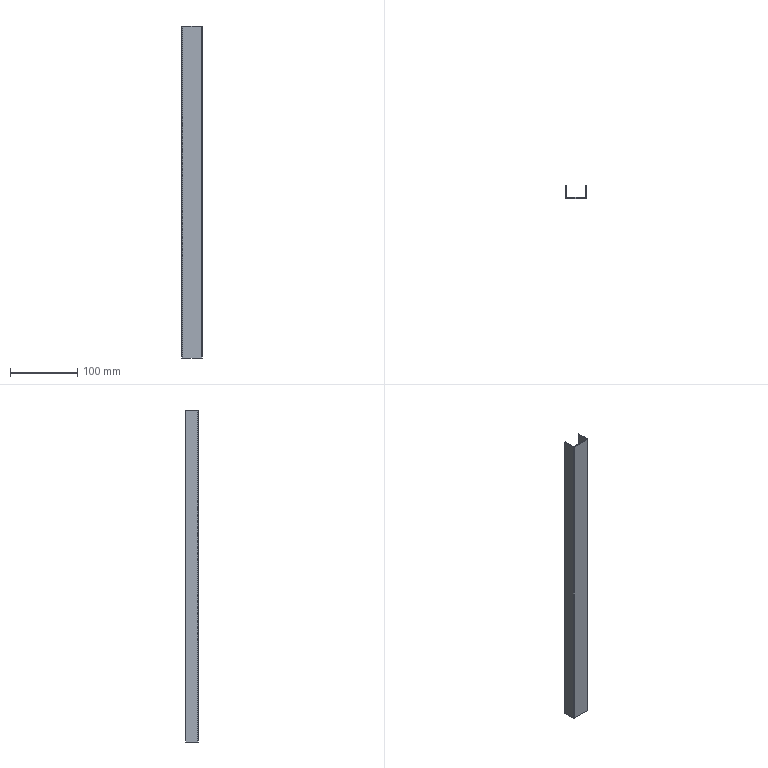Part | SolidWorks | features SplitBody 1 | 1 solid | 22 faces | box 30 x 19 x 495 mm | volume 32415 mm3 | plane 18 | cylinder 4 | commonest cylinder face diameters 0.2 x2 2.2 x2
STEP:
#1=CARTESIAN_POINT('',(-13.9,1595.5,-247.5));
#2=VERTEX_POINT('',#1);
#3=CARTESIAN_POINT('',(-13.9,1596.5,-247.5));
#4=VERTEX_POINT('',#3);
#5=CARTESIAN_POINT('',(-13.9,1595.5,-247.5));
#6=DIRECTION('',(0.,1.,0.));
#7=VECTOR('',#6,1000.);
#8=LINE('',#5,#7);
#9=EDGE_CURVE('',#2,#4,#8,.T.);
#10=ORIENTED_EDGE('',*,*,#9,.F.);
#11=CARTESIAN_POINT('',(-15.,1596.6,-247.5));
#12=VERTEX_POINT('',#11);
#13=CARTESIAN_POINT('',(-13.9,1596.6,-247.5));
#14=DIRECTION('',(0.,0.,1.));
#15=DIRECTION('',(-1.,0.,0.));
#16=AXIS2_PLACEMENT_3D('',#13,#14,#15);
#17=CIRCLE('',#16,1.1);
#18=EDGE_CURVE('',#12,#2,#17,.T.);
#19=ORIENTED_EDGE('',*,*,#18,.F.);
#20=CARTESIAN_POINT('',(-14.,1596.6,-247.5));
#21=VERTEX_POINT('',#20);
#22=CARTESIAN_POINT('',(-14.,1596.6,-247.5));
#23=DIRECTION('',(-1.,0.,0.));
#24=VECTOR('',#23,1000.);
#25=LINE('',#22,#24);
#26=EDGE_CURVE('',#21,#12,#25,.T.);
#27=ORIENTED_EDGE('',*,*,#26,.F.);
#28=CARTESIAN_POINT('',(-13.9,1596.6,-247.5));
#29=DIRECTION('',(0.,0.,1.));
#30=DIRECTION('',(1.,0.,0.));
#31=AXIS2_PLACEMENT_3D('',#28,#29,#30);
#32=CIRCLE('',#31,0.1);
#33=EDGE_CURVE('',#21,#4,#32,.T.);
#34=ORIENTED_EDGE('',*,*,#33,.T.);
#35=EDGE_LOOP('',(#10,#19,#27,#34));
#36=FACE_OUTER_BOUND('',#35,.T.);
#37=CARTESIAN_POINT('',(-13.9,1595.5,-247.5));
#38=DIRECTION('',(0.,0.,-1.));
#39=DIRECTION('',(-1.,0.,0.));
#40=AXIS2_PLACEMENT_3D('',#37,#38,#39);
#41=PLANE('',#40);
#42=ADVANCED_FACE('',(#36),#41,.T.);
#43=CARTESIAN_POINT('',(13.9,1595.5,-247.5));
#44=VERTEX_POINT('',#43);
#45=CARTESIAN_POINT('',(-15.,1595.5,-247.5));
#46=DIRECTION('',(1.,0.,0.));
#47=VECTOR('',#46,1000.);
#48=LINE('',#45,#47);
#49=EDGE_CURVE('',#2,#44,#48,.T.);
#50=ORIENTED_EDGE('',*,*,#49,.F.);
#51=ORIENTED_EDGE('',*,*,#9,.T.);
#52=CARTESIAN_POINT('',(13.9,1596.5,-247.5));
#53=VERTEX_POINT('',#52);
#54=CARTESIAN_POINT('',(-15.,1596.5,-247.5));
#55=DIRECTION('',(1.,0.,0.));
#56=VECTOR('',#55,1000.);
#57=LINE('',#54,#56);
#58=EDGE_CURVE('',#4,#53,#57,.T.);
#59=ORIENTED_EDGE('',*,*,#58,.T.);
#60=CARTESIAN_POINT('',(13.9,1596.5,-247.5));
#61=DIRECTION('',(0.,-1.,0.));
#62=VECTOR('',#61,1000.);
#63=LINE('',#60,#62);
#64=EDGE_CURVE('',#53,#44,#63,.T.);
#65=ORIENTED_EDGE('',*,*,#64,.T.);
#66=EDGE_LOOP('',(#50,#51,#59,#65));
#67=FACE_OUTER_BOUND('',#66,.T.);
#68=CARTESIAN_POINT('',(-14.,1596.6,-247.5));
#69=DIRECTION('',(0.,0.,-1.));
#70=DIRECTION('',(-1.,0.,0.));
#71=AXIS2_PLACEMENT_3D('',#68,#69,#70);
#72=PLANE('',#71);
#73=ADVANCED_FACE('',(#67),#72,.T.);
#74=CARTESIAN_POINT('',(15.,1596.6,-247.5));
#75=VERTEX_POINT('',#74);
#76=CARTESIAN_POINT('',(14.,1596.6,-247.5));
#77=VERTEX_POINT('',#76);
#78=CARTESIAN_POINT('',(15.,1596.6,-247.5));
#79=DIRECTION('',(-1.,0.,0.));
#80=VECTOR('',#79,1000.);
#81=LINE('',#78,#80);
#82=EDGE_CURVE('',#75,#77,#81,.T.);
#83=ORIENTED_EDGE('',*,*,#82,.F.);
#84=CARTESIAN_POINT('',(13.9,1596.6,-247.5));
#85=DIRECTION('',(0.,0.,1.));
#86=DIRECTION('',(-1.,0.,0.));
#87=AXIS2_PLACEMENT_3D('',#84,#85,#86);
#88=CIRCLE('',#87,1.1);
#89=EDGE_CURVE('',#44,#75,#88,.T.);
#90=ORIENTED_EDGE('',*,*,#89,.F.);
#91=ORIENTED_EDGE('',*,*,#64,.F.);
#92=CARTESIAN_POINT('',(13.9,1596.6,-247.5));
#93=DIRECTION('',(0.,0.,1.));
#94=DIRECTION('',(1.,0.,0.));
#95=AXIS2_PLACEMENT_3D('',#92,#93,#94);
#96=CIRCLE('',#95,0.1);
#97=EDGE_CURVE('',#53,#77,#96,.T.);
#98=ORIENTED_EDGE('',*,*,#97,.T.);
#99=EDGE_LOOP('',(#83,#90,#91,#98));
#100=FACE_OUTER_BOUND('',#99,.T.);
#101=CARTESIAN_POINT('',(15.,1596.6,-247.5));
#102=DIRECTION('',(0.,0.,-1.));
#103=DIRECTION('',(-1.,0.,0.));
#104=AXIS2_PLACEMENT_3D('',#101,#102,#103);
#105=PLANE('',#104);
#106=ADVANCED_FACE('',(#100),#105,.T.);
#107=CARTESIAN_POINT('',(15.,1614.5,-247.5));
#108=VERTEX_POINT('',#107);
#109=CARTESIAN_POINT('',(15.,1595.5,-247.5));
#110=DIRECTION('',(0.,1.,0.));
#111=VECTOR('',#110,1000.);
#112=LINE('',#109,#111);
#113=EDGE_CURVE('',#75,#108,#112,.T.);
#114=ORIENTED_EDGE('',*,*,#113,.F.);
#115=ORIENTED_EDGE('',*,*,#82,.T.);
#116=CARTESIAN_POINT('',(14.,1614.5,-247.5));
#117=VERTEX_POINT('',#116);
#118=CARTESIAN_POINT('',(14.,1595.5,-247.5));
#119=DIRECTION('',(0.,1.,0.));
#120=VECTOR('',#119,1000.);
#121=LINE('',#118,#120);
#122=EDGE_CURVE('',#77,#117,#121,.T.);
#123=ORIENTED_EDGE('',*,*,#122,.T.);
#124=CARTESIAN_POINT('',(14.,1614.5,-247.5));
#125=DIRECTION('',(1.,0.,0.));
#126=VECTOR('',#125,1000.);
#127=LINE('',#124,#126);
#128=EDGE_CURVE('',#117,#108,#127,.T.);
#129=ORIENTED_EDGE('',*,*,#128,.T.);
#130=EDGE_LOOP('',(#114,#115,#123,#129));
#131=FACE_OUTER_BOUND('',#130,.T.);
#132=CARTESIAN_POINT('',(13.9,1596.5,-247.5));
#133=DIRECTION('',(0.,0.,-1.));
#134=DIRECTION('',(-1.,0.,0.));
#135=AXIS2_PLACEMENT_3D('',#132,#133,#134);
#136=PLANE('',#135);
#137=ADVANCED_FACE('',(#131),#136,.T.);
#138=CARTESIAN_POINT('',(15.,1614.5,247.5));
#139=VERTEX_POINT('',#138);
#140=CARTESIAN_POINT('',(15.,1596.6,247.5));
#141=VERTEX_POINT('',#140);
#142=CARTESIAN_POINT('',(15.,1595.5,247.5));
#143=DIRECTION('',(0.,-1.,0.));
#144=VECTOR('',#143,1000.);
#145=LINE('',#142,#144);
#146=EDGE_CURVE('',#139,#141,#145,.T.);
#147=ORIENTED_EDGE('',*,*,#146,.T.);
#148=CARTESIAN_POINT('',(15.,1596.6,283.011));
#149=DIRECTION('',(0.,0.,-1.));
#150=VECTOR('',#149,1000.);
#151=LINE('',#148,#150);
#152=EDGE_CURVE('',#141,#75,#151,.T.);
#153=ORIENTED_EDGE('',*,*,#152,.T.);
#154=ORIENTED_EDGE('',*,*,#113,.T.);
#155=CARTESIAN_POINT('',(15.,1614.5,283.011));
#156=DIRECTION('',(0.,0.,-1.));
#157=VECTOR('',#156,1000.);
#158=LINE('',#155,#157);
#159=EDGE_CURVE('',#139,#108,#158,.T.);
#160=ORIENTED_EDGE('',*,*,#159,.F.);
#161=EDGE_LOOP('',(#147,#153,#154,#160));
#162=FACE_OUTER_BOUND('',#161,.T.);
#163=CARTESIAN_POINT('',(15.,1595.5,283.011));
#164=DIRECTION('',(-1.,0.,0.));
#165=DIRECTION('',(0.,-1.,0.));
#166=AXIS2_PLACEMENT_3D('',#163,#164,#165);
#167=PLANE('',#166);
#168=ADVANCED_FACE('',(#162),#167,.F.);
#169=CARTESIAN_POINT('',(14.,1614.5,247.5));
#170=VERTEX_POINT('',#169);
#171=CARTESIAN_POINT('',(14.,1614.5,283.011));
#172=DIRECTION('',(0.,0.,-1.));
#173=VECTOR('',#172,1000.);
#174=LINE('',#171,#173);
#175=EDGE_CURVE('',#170,#117,#174,.T.);
#176=ORIENTED_EDGE('',*,*,#175,.F.);
#177=CARTESIAN_POINT('',(15.,1614.5,247.5));
#178=DIRECTION('',(-1.,0.,0.));
#179=VECTOR('',#178,1000.);
#180=LINE('',#177,#179);
#181=EDGE_CURVE('',#139,#170,#180,.T.);
#182=ORIENTED_EDGE('',*,*,#181,.F.);
#183=ORIENTED_EDGE('',*,*,#159,.T.);
#184=ORIENTED_EDGE('',*,*,#128,.F.);
#185=EDGE_LOOP('',(#176,#182,#183,#184));
#186=FACE_OUTER_BOUND('',#185,.T.);
#187=CARTESIAN_POINT('',(14.,1614.5,283.011));
#188=DIRECTION('',(0.,1.,0.));
#189=DIRECTION('',(0.,0.,1.));
#190=AXIS2_PLACEMENT_3D('',#187,#188,#189);
#191=PLANE('',#190);
#192=ADVANCED_FACE('',(#186),#191,.T.);
#193=CARTESIAN_POINT('',(14.,1596.6,247.5));
#194=VERTEX_POINT('',#193);
#195=CARTESIAN_POINT('',(14.,1596.6,283.011));
#196=DIRECTION('',(0.,0.,-1.));
#197=VECTOR('',#196,1000.);
#198=LINE('',#195,#197);
#199=EDGE_CURVE('',#194,#77,#198,.T.);
#200=ORIENTED_EDGE('',*,*,#199,.F.);
#201=CARTESIAN_POINT('',(14.,1595.5,247.5));
#202=DIRECTION('',(0.,-1.,0.));
#203=VECTOR('',#202,1000.);
#204=LINE('',#201,#203);
#205=EDGE_CURVE('',#170,#194,#204,.T.);
#206=ORIENTED_EDGE('',*,*,#205,.F.);
#207=ORIENTED_EDGE('',*,*,#175,.T.);
#208=ORIENTED_EDGE('',*,*,#122,.F.);
#209=EDGE_LOOP('',(#200,#206,#207,#208));
#210=FACE_OUTER_BOUND('',#209,.T.);
#211=CARTESIAN_POINT('',(14.,1595.5,283.011));
#212=DIRECTION('',(-1.,0.,0.));
#213=DIRECTION('',(0.,-1.,0.));
#214=AXIS2_PLACEMENT_3D('',#211,#212,#213);
#215=PLANE('',#214);
#216=ADVANCED_FACE('',(#210),#215,.T.);
#217=CARTESIAN_POINT('',(13.9,1596.5,247.5));
#218=VERTEX_POINT('',#217);
#219=CARTESIAN_POINT('',(13.9,1596.5,283.011));
#220=DIRECTION('',(0.,0.,-1.));
#221=VECTOR('',#220,1000.);
#222=LINE('',#219,#221);
#223=EDGE_CURVE('',#218,#53,#222,.T.);
#224=ORIENTED_EDGE('',*,*,#223,.F.);
#225=CARTESIAN_POINT('',(13.9,1596.6,247.5));
#226=DIRECTION('',(0.,0.,-1.));
#227=DIRECTION('',(1.,0.,0.));
#228=AXIS2_PLACEMENT_3D('',#225,#226,#227);
#229=CIRCLE('',#228,0.1);
#230=EDGE_CURVE('',#194,#218,#229,.T.);
#231=ORIENTED_EDGE('',*,*,#230,.F.);
#232=ORIENTED_EDGE('',*,*,#199,.T.);
#233=ORIENTED_EDGE('',*,*,#97,.F.);
#234=EDGE_LOOP('',(#224,#231,#232,#233));
#235=FACE_OUTER_BOUND('',#234,.T.);
#236=CARTESIAN_POINT('',(13.9,1596.6,283.011));
#237=DIRECTION('',(0.,0.,-1.));
#238=DIRECTION('',(-1.,0.,0.));
#239=AXIS2_PLACEMENT_3D('',#236,#237,#238);
#240=CYLINDRICAL_SURFACE('',#239,0.1);
#241=ADVANCED_FACE('',(#235),#240,.F.);
#242=CARTESIAN_POINT('',(-13.9,1596.5,247.5));
#243=VERTEX_POINT('',#242);
#244=CARTESIAN_POINT('',(-13.9,1596.5,283.011));
#245=DIRECTION('',(0.,0.,-1.));
#246=VECTOR('',#245,1000.);
#247=LINE('',#244,#246);
#248=EDGE_CURVE('',#243,#4,#247,.T.);
#249=ORIENTED_EDGE('',*,*,#248,.F.);
#250=CARTESIAN_POINT('',(-15.,1596.5,247.5));
#251=DIRECTION('',(-1.,0.,0.));
#252=VECTOR('',#251,1000.);
#253=LINE('',#250,#252);
#254=EDGE_CURVE('',#218,#243,#253,.T.);
#255=ORIENTED_EDGE('',*,*,#254,.F.);
#256=ORIENTED_EDGE('',*,*,#223,.T.);
#257=ORIENTED_EDGE('',*,*,#58,.F.);
#258=EDGE_LOOP('',(#249,#255,#256,#257));
#259=FACE_OUTER_BOUND('',#258,.T.);
#260=CARTESIAN_POINT('',(-15.,1596.5,283.011));
#261=DIRECTION('',(0.,1.,0.));
#262=DIRECTION('',(0.,0.,1.));
#263=AXIS2_PLACEMENT_3D('',#260,#261,#262);
#264=PLANE('',#263);
#265=ADVANCED_FACE('',(#259),#264,.T.);
#266=CARTESIAN_POINT('',(-14.,1596.6,247.5));
#267=VERTEX_POINT('',#266);
#268=CARTESIAN_POINT('',(-14.,1596.6,283.011));
#269=DIRECTION('',(0.,0.,-1.));
#270=VECTOR('',#269,1000.);
#271=LINE('',#268,#270);
#272=EDGE_CURVE('',#267,#21,#271,.T.);
#273=ORIENTED_EDGE('',*,*,#272,.F.);
#274=CARTESIAN_POINT('',(-13.9,1596.6,247.5));
#275=DIRECTION('',(0.,0.,-1.));
#276=DIRECTION('',(1.,0.,0.));
#277=AXIS2_PLACEMENT_3D('',#274,#275,#276);
#278=CIRCLE('',#277,0.1);
#279=EDGE_CURVE('',#243,#267,#278,.T.);
#280=ORIENTED_EDGE('',*,*,#279,.F.);
#281=ORIENTED_EDGE('',*,*,#248,.T.);
#282=ORIENTED_EDGE('',*,*,#33,.F.);
#283=EDGE_LOOP('',(#273,#280,#281,#282));
#284=FACE_OUTER_BOUND('',#283,.T.);
#285=CARTESIAN_POINT('',(-13.9,1596.6,283.011));
#286=DIRECTION('',(0.,0.,-1.));
#287=DIRECTION('',(-1.,0.,0.));
#288=AXIS2_PLACEMENT_3D('',#285,#286,#287);
#289=CYLINDRICAL_SURFACE('',#288,0.1);
#290=ADVANCED_FACE('',(#284),#289,.F.);
#291=CARTESIAN_POINT('',(-14.,1614.5,247.5));
#292=VERTEX_POINT('',#291);
#293=CARTESIAN_POINT('',(-14.,1614.5,-247.5));
#294=VERTEX_POINT('',#293);
#295=CARTESIAN_POINT('',(-14.,1614.5,283.011));
#296=DIRECTION('',(0.,0.,-1.));
#297=VECTOR('',#296,1000.);
#298=LINE('',#295,#297);
#299=EDGE_CURVE('',#292,#294,#298,.T.);
#300=ORIENTED_EDGE('',*,*,#299,.F.);
#301=CARTESIAN_POINT('',(-14.,1614.5,247.5));
#302=DIRECTION('',(0.,1.,0.));
#303=VECTOR('',#302,1000.);
#304=LINE('',#301,#303);
#305=EDGE_CURVE('',#267,#292,#304,.T.);
#306=ORIENTED_EDGE('',*,*,#305,.F.);
#307=ORIENTED_EDGE('',*,*,#272,.T.);
#308=CARTESIAN_POINT('',(-14.,1614.5,-247.5));
#309=DIRECTION('',(0.,-1.,0.));
#310=VECTOR('',#309,1000.);
#311=LINE('',#308,#310);
#312=EDGE_CURVE('',#294,#21,#311,.T.);
#313=ORIENTED_EDGE('',*,*,#312,.F.);
#314=EDGE_LOOP('',(#300,#306,#307,#313));
#315=FACE_OUTER_BOUND('',#314,.T.);
#316=CARTESIAN_POINT('',(-14.,1614.5,283.011));
#317=DIRECTION('',(1.,0.,0.));
#318=DIRECTION('',(0.,1.,0.));
#319=AXIS2_PLACEMENT_3D('',#316,#317,#318);
#320=PLANE('',#319);
#321=ADVANCED_FACE('',(#315),#320,.T.);
#322=CARTESIAN_POINT('',(-15.,1614.5,247.5));
#323=VERTEX_POINT('',#322);
#324=CARTESIAN_POINT('',(-15.,1614.5,-247.5));
#325=VERTEX_POINT('',#324);
#326=CARTESIAN_POINT('',(-15.,1614.5,283.011));
#327=DIRECTION('',(0.,0.,-1.));
#328=VECTOR('',#327,1000.);
#329=LINE('',#326,#328);
#330=EDGE_CURVE('',#323,#325,#329,.T.);
#331=ORIENTED_EDGE('',*,*,#330,.F.);
#332=CARTESIAN_POINT('',(-15.,1614.5,247.5));
#333=DIRECTION('',(1.,0.,0.));
#334=VECTOR('',#333,1000.);
#335=LINE('',#332,#334);
#336=EDGE_CURVE('',#323,#292,#335,.T.);
#337=ORIENTED_EDGE('',*,*,#336,.T.);
#338=ORIENTED_EDGE('',*,*,#299,.T.);
#339=CARTESIAN_POINT('',(-15.,1614.5,-247.5));
#340=DIRECTION('',(1.,0.,0.));
#341=VECTOR('',#340,1000.);
#342=LINE('',#339,#341);
#343=EDGE_CURVE('',#325,#294,#342,.T.);
#344=ORIENTED_EDGE('',*,*,#343,.F.);
#345=EDGE_LOOP('',(#331,#337,#338,#344));
#346=FACE_OUTER_BOUND('',#345,.T.);
#347=CARTESIAN_POINT('',(-15.,1614.5,283.011));
#348=DIRECTION('',(0.,1.,0.));
#349=DIRECTION('',(0.,0.,1.));
#350=AXIS2_PLACEMENT_3D('',#347,#348,#349);
#351=PLANE('',#350);
#352=ADVANCED_FACE('',(#346),#351,.T.);
#353=CARTESIAN_POINT('',(-15.,1596.6,247.5));
#354=VERTEX_POINT('',#353);
#355=CARTESIAN_POINT('',(-15.,1614.5,247.5));
#356=DIRECTION('',(0.,1.,0.));
#357=VECTOR('',#356,1000.);
#358=LINE('',#355,#357);
#359=EDGE_CURVE('',#354,#323,#358,.T.);
#360=ORIENTED_EDGE('',*,*,#359,.T.);
#361=ORIENTED_EDGE('',*,*,#330,.T.);
#362=CARTESIAN_POINT('',(-15.,1614.5,-247.5));
#363=DIRECTION('',(0.,-1.,0.));
#364=VECTOR('',#363,1000.);
#365=LINE('',#362,#364);
#366=EDGE_CURVE('',#325,#12,#365,.T.);
#367=ORIENTED_EDGE('',*,*,#366,.T.);
#368=CARTESIAN_POINT('',(-15.,1596.6,283.011));
#369=DIRECTION('',(0.,0.,-1.));
#370=VECTOR('',#369,1000.);
#371=LINE('',#368,#370);
#372=EDGE_CURVE('',#354,#12,#371,.T.);
#373=ORIENTED_EDGE('',*,*,#372,.F.);
#374=EDGE_LOOP('',(#360,#361,#367,#373));
#375=FACE_OUTER_BOUND('',#374,.T.);
#376=CARTESIAN_POINT('',(-15.,1614.5,283.011));
#377=DIRECTION('',(1.,0.,0.));
#378=DIRECTION('',(0.,1.,0.));
#379=AXIS2_PLACEMENT_3D('',#376,#377,#378);
#380=PLANE('',#379);
#381=ADVANCED_FACE('',(#375),#380,.F.);
#382=CARTESIAN_POINT('',(-13.9,1595.5,247.5));
#383=VERTEX_POINT('',#382);
#384=CARTESIAN_POINT('',(-13.9,1596.6,247.5));
#385=DIRECTION('',(0.,0.,-1.));
#386=DIRECTION('',(-1.,0.,0.));
#387=AXIS2_PLACEMENT_3D('',#384,#385,#386);
#388=CIRCLE('',#387,1.1);
#389=EDGE_CURVE('',#383,#354,#388,.T.);
#390=ORIENTED_EDGE('',*,*,#389,.T.);
#391=ORIENTED_EDGE('',*,*,#372,.T.);
#392=ORIENTED_EDGE('',*,*,#18,.T.);
#393=CARTESIAN_POINT('',(-13.9,1595.5,283.011));
#394=DIRECTION('',(0.,0.,-1.));
#395=VECTOR('',#394,1000.);
#396=LINE('',#393,#395);
#397=EDGE_CURVE('',#383,#2,#396,.T.);
#398=ORIENTED_EDGE('',*,*,#397,.F.);
#399=EDGE_LOOP('',(#390,#391,#392,#398));
#400=FACE_OUTER_BOUND('',#399,.T.);
#401=CARTESIAN_POINT('',(-13.9,1596.6,283.011));
#402=DIRECTION('',(0.,0.,-1.));
#403=DIRECTION('',(-1.,0.,0.));
#404=AXIS2_PLACEMENT_3D('',#401,#402,#403);
#405=CYLINDRICAL_SURFACE('',#404,1.1);
#406=ADVANCED_FACE('',(#400),#405,.T.);
#407=CARTESIAN_POINT('',(13.9,1595.5,247.5));
#408=VERTEX_POINT('',#407);
#409=CARTESIAN_POINT('',(-15.,1595.5,247.5));
#410=DIRECTION('',(-1.,0.,0.));
#411=VECTOR('',#410,1000.);
#412=LINE('',#409,#411);
#413=EDGE_CURVE('',#408,#383,#412,.T.);
#414=ORIENTED_EDGE('',*,*,#413,.T.);
#415=ORIENTED_EDGE('',*,*,#397,.T.);
#416=ORIENTED_EDGE('',*,*,#49,.T.);
#417=CARTESIAN_POINT('',(13.9,1595.5,283.011));
#418=DIRECTION('',(0.,0.,-1.));
#419=VECTOR('',#418,1000.);
#420=LINE('',#417,#419);
#421=EDGE_CURVE('',#408,#44,#420,.T.);
#422=ORIENTED_EDGE('',*,*,#421,.F.);
#423=EDGE_LOOP('',(#414,#415,#416,#422));
#424=FACE_OUTER_BOUND('',#423,.T.);
#425=CARTESIAN_POINT('',(-15.,1595.5,283.011));
#426=DIRECTION('',(0.,1.,0.));
#427=DIRECTION('',(0.,0.,1.));
#428=AXIS2_PLACEMENT_3D('',#425,#426,#427);
#429=PLANE('',#428);
#430=ADVANCED_FACE('',(#424),#429,.F.);
#431=CARTESIAN_POINT('',(13.9,1596.6,247.5));
#432=DIRECTION('',(0.,0.,-1.));
#433=DIRECTION('',(-1.,0.,0.));
#434=AXIS2_PLACEMENT_3D('',#431,#432,#433);
#435=CIRCLE('',#434,1.1);
#436=EDGE_CURVE('',#141,#408,#435,.T.);
#437=ORIENTED_EDGE('',*,*,#436,.T.);
#438=ORIENTED_EDGE('',*,*,#421,.T.);
#439=ORIENTED_EDGE('',*,*,#89,.T.);
#440=ORIENTED_EDGE('',*,*,#152,.F.);
#441=EDGE_LOOP('',(#437,#438,#439,#440));
#442=FACE_OUTER_BOUND('',#441,.T.);
#443=CARTESIAN_POINT('',(13.9,1596.6,283.011));
#444=DIRECTION('',(0.,0.,-1.));
#445=DIRECTION('',(-1.,0.,0.));
#446=AXIS2_PLACEMENT_3D('',#443,#444,#445);
#447=CYLINDRICAL_SURFACE('',#446,1.1);
#448=ADVANCED_FACE('',(#442),#447,.T.);
#449=ORIENTED_EDGE('',*,*,#312,.T.);
#450=ORIENTED_EDGE('',*,*,#26,.T.);
#451=ORIENTED_EDGE('',*,*,#366,.F.);
#452=ORIENTED_EDGE('',*,*,#343,.T.);
#453=EDGE_LOOP('',(#449,#450,#451,#452));
#454=FACE_OUTER_BOUND('',#453,.T.);
#455=CARTESIAN_POINT('',(13.9,1596.6,-247.5));
#456=DIRECTION('',(0.,0.,1.));
#457=DIRECTION('',(1.,0.,0.));
#458=AXIS2_PLACEMENT_3D('',#455,#456,#457);
#459=PLANE('',#458);
#460=ADVANCED_FACE('',(#454),#459,.F.);
#461=CARTESIAN_POINT('',(15.,1596.6,247.5));
#462=DIRECTION('',(-1.,0.,0.));
#463=VECTOR('',#462,1000.);
#464=LINE('',#461,#463);
#465=EDGE_CURVE('',#141,#194,#464,.T.);
#466=ORIENTED_EDGE('',*,*,#465,.F.);
#467=ORIENTED_EDGE('',*,*,#146,.F.);
#468=ORIENTED_EDGE('',*,*,#181,.T.);
#469=ORIENTED_EDGE('',*,*,#205,.T.);
#470=EDGE_LOOP('',(#466,#467,#468,#469));
#471=FACE_OUTER_BOUND('',#470,.T.);
#472=CARTESIAN_POINT('',(15.,1595.5,247.5));
#473=DIRECTION('',(0.,0.,-1.));
#474=DIRECTION('',(0.,-1.,0.));
#475=AXIS2_PLACEMENT_3D('',#472,#473,#474);
#476=PLANE('',#475);
#477=ADVANCED_FACE('',(#471),#476,.F.);
#478=CARTESIAN_POINT('',(-13.9,1595.5,247.5));
#479=DIRECTION('',(0.,1.,0.));
#480=VECTOR('',#479,1000.);
#481=LINE('',#478,#480);
#482=EDGE_CURVE('',#383,#243,#481,.T.);
#483=ORIENTED_EDGE('',*,*,#482,.F.);
#484=ORIENTED_EDGE('',*,*,#413,.F.);
#485=CARTESIAN_POINT('',(13.9,1595.5,247.5));
#486=DIRECTION('',(0.,1.,0.));
#487=VECTOR('',#486,1000.);
#488=LINE('',#485,#487);
#489=EDGE_CURVE('',#408,#218,#488,.T.);
#490=ORIENTED_EDGE('',*,*,#489,.T.);
#491=ORIENTED_EDGE('',*,*,#254,.T.);
#492=EDGE_LOOP('',(#483,#484,#490,#491));
#493=FACE_OUTER_BOUND('',#492,.T.);
#494=CARTESIAN_POINT('',(-15.,1595.5,247.5));
#495=DIRECTION('',(0.,0.,-1.));
#496=DIRECTION('',(-1.,0.,0.));
#497=AXIS2_PLACEMENT_3D('',#494,#495,#496);
#498=PLANE('',#497);
#499=ADVANCED_FACE('',(#493),#498,.F.);
#500=ORIENTED_EDGE('',*,*,#336,.F.);
#501=ORIENTED_EDGE('',*,*,#359,.F.);
#502=CARTESIAN_POINT('',(-15.,1596.6,247.5));
#503=DIRECTION('',(1.,0.,0.));
#504=VECTOR('',#503,1000.);
#505=LINE('',#502,#504);
#506=EDGE_CURVE('',#354,#267,#505,.T.);
#507=ORIENTED_EDGE('',*,*,#506,.T.);
#508=ORIENTED_EDGE('',*,*,#305,.T.);
#509=EDGE_LOOP('',(#500,#501,#507,#508));
#510=FACE_OUTER_BOUND('',#509,.T.);
#511=CARTESIAN_POINT('',(-15.,1614.5,247.5));
#512=DIRECTION('',(0.,0.,-1.));
#513=DIRECTION('',(0.,1.,0.));
#514=AXIS2_PLACEMENT_3D('',#511,#512,#513);
#515=PLANE('',#514);
#516=ADVANCED_FACE('',(#510),#515,.F.);
#517=ORIENTED_EDGE('',*,*,#279,.T.);
#518=ORIENTED_EDGE('',*,*,#506,.F.);
#519=ORIENTED_EDGE('',*,*,#389,.F.);
#520=ORIENTED_EDGE('',*,*,#482,.T.);
#521=EDGE_LOOP('',(#517,#518,#519,#520));
#522=FACE_OUTER_BOUND('',#521,.T.);
#523=CARTESIAN_POINT('',(-13.9,1596.6,247.5));
#524=DIRECTION('',(0.,0.,1.));
#525=DIRECTION('',(1.,0.,0.));
#526=AXIS2_PLACEMENT_3D('',#523,#524,#525);
#527=PLANE('',#526);
#528=ADVANCED_FACE('',(#522),#527,.T.);
#529=ORIENTED_EDGE('',*,*,#230,.T.);
#530=ORIENTED_EDGE('',*,*,#489,.F.);
#531=ORIENTED_EDGE('',*,*,#436,.F.);
#532=ORIENTED_EDGE('',*,*,#465,.T.);
#533=EDGE_LOOP('',(#529,#530,#531,#532));
#534=FACE_OUTER_BOUND('',#533,.T.);
#535=CARTESIAN_POINT('',(13.9,1596.6,247.5));
#536=DIRECTION('',(0.,0.,1.));
#537=DIRECTION('',(1.,0.,0.));
#538=AXIS2_PLACEMENT_3D('',#535,#536,#537);
#539=PLANE('',#538);
#540=ADVANCED_FACE('',(#534),#539,.T.);
#541=CLOSED_SHELL('',(#42,#73,#106,#137,#168,#192,#216,#241,#265,#290,#321,#352,#381,#406,#430,#448,#460,#477,#499,#516,#528,#540));
#542=MANIFOLD_SOLID_BREP('',#541);
#543=CARTESIAN_POINT('',(0.,0.,0.));
#544=DIRECTION('',(0.,0.,1.));
#545=DIRECTION('',(1.,0.,0.));
#546=AXIS2_PLACEMENT_3D('',#543,#544,#545);
#547=(LENGTH_UNIT()NAMED_UNIT(*)SI_UNIT(.MILLI.,.METRE.));
#548=UNCERTAINTY_MEASURE_WITH_UNIT(LENGTH_MEASURE(0.00001),#547,'','');
#549=(NAMED_UNIT(*)PLANE_ANGLE_UNIT()SI_UNIT($,.RADIAN.));
#550=(NAMED_UNIT(*)SI_UNIT($,.STERADIAN.)SOLID_ANGLE_UNIT());
#551=(GEOMETRIC_REPRESENTATION_CONTEXT(3)GLOBAL_UNCERTAINTY_ASSIGNED_CONTEXT((#548))GLOBAL_UNIT_ASSIGNED_CONTEXT((#547,#549,#550))REPRESENTATION_CONTEXT('',''));
#552=ADVANCED_BREP_SHAPE_REPRESENTATION('',(#542,#546),#551);